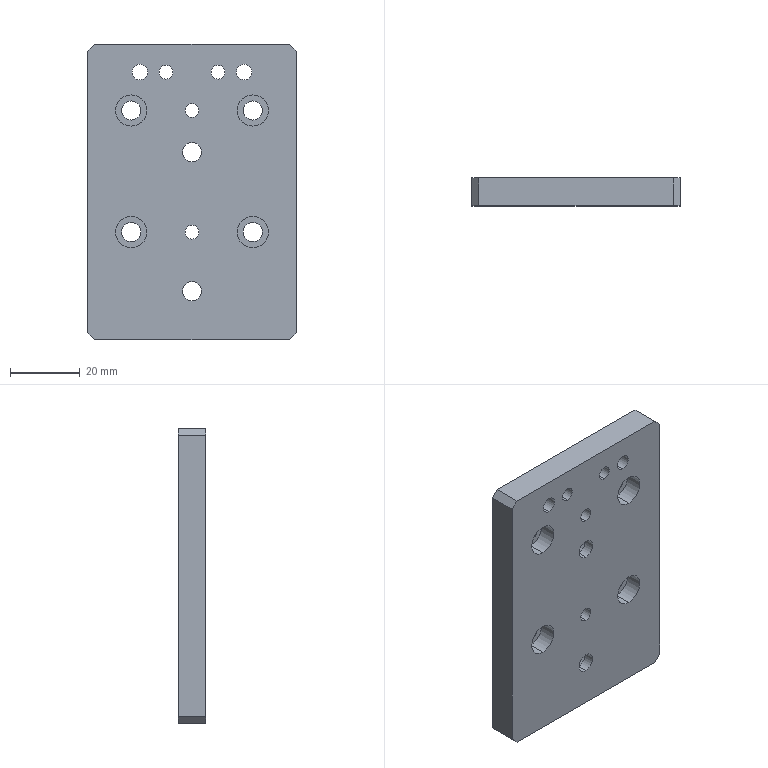Part | SolidWorks | features HoleWzd 4, Chamfer 1, Extrusion 1 | 1 solid | 58 faces | box 60 x 8 x 85 mm | volume 37427 mm3 | cylinder 40 | plane 18 | commonest cylinder face diameters 5.5 x12 9 x12 4 x8 4.5 x4 8 x4